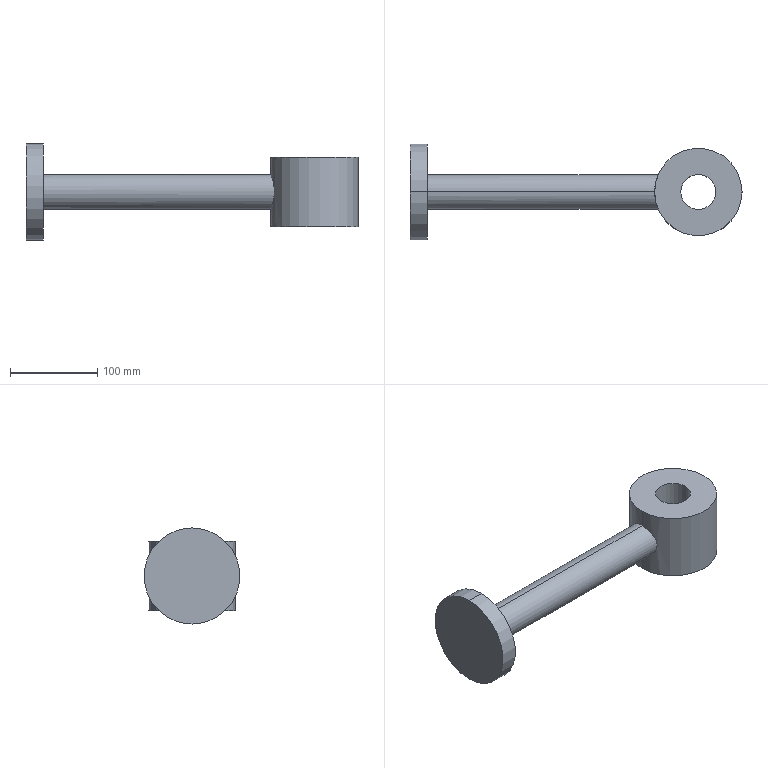Part | SolidWorks | 1 solid | 12 faces | box 380 x 110 x 110 mm | volume 1045872 mm3 | cylinder 8 | plane 4 | commonest cylinder face diameters 40 x4 100 x2 110 x2
STEP:
#1=CARTESIAN_POINT('',(310.,0.,40.));
#2=VERTEX_POINT('',#1);
#3=CARTESIAN_POINT('',(350.,0.,40.));
#4=VERTEX_POINT('',#3);
#5=CARTESIAN_POINT('',(330.,0.,40.));
#6=DIRECTION('',(0.,0.,1.));
#7=DIRECTION('',(1.,0.,0.));
#8=AXIS2_PLACEMENT_3D('',#5,#6,#7);
#9=CIRCLE('',#8,20.);
#10=EDGE_CURVE('',#2,#4,#9,.T.);
#11=ORIENTED_EDGE('',*,*,#10,.T.);
#12=CARTESIAN_POINT('',(350.,0.,-40.));
#13=VERTEX_POINT('',#12);
#14=CARTESIAN_POINT('',(350.,0.,40.));
#15=DIRECTION('',(0.,0.,-1.));
#16=VECTOR('',#15,1000.);
#17=LINE('',#14,#16);
#18=EDGE_CURVE('',#4,#13,#17,.T.);
#19=ORIENTED_EDGE('',*,*,#18,.T.);
#20=CARTESIAN_POINT('',(310.,0.,-40.));
#21=VERTEX_POINT('',#20);
#22=CARTESIAN_POINT('',(330.,0.,-40.));
#23=DIRECTION('',(0.,0.,1.));
#24=DIRECTION('',(1.,0.,0.));
#25=AXIS2_PLACEMENT_3D('',#22,#23,#24);
#26=CIRCLE('',#25,20.);
#27=EDGE_CURVE('',#21,#13,#26,.T.);
#28=ORIENTED_EDGE('',*,*,#27,.F.);
#29=CARTESIAN_POINT('',(310.,0.,40.));
#30=DIRECTION('',(0.,0.,-1.));
#31=VECTOR('',#30,1000.);
#32=LINE('',#29,#31);
#33=EDGE_CURVE('',#2,#21,#32,.T.);
#34=ORIENTED_EDGE('',*,*,#33,.F.);
#35=EDGE_LOOP('',(#11,#19,#28,#34));
#36=FACE_OUTER_BOUND('',#35,.T.);
#37=CARTESIAN_POINT('',(330.,0.,40.));
#38=DIRECTION('',(0.,0.,-1.));
#39=DIRECTION('',(-1.,0.,0.));
#40=AXIS2_PLACEMENT_3D('',#37,#38,#39);
#41=CYLINDRICAL_SURFACE('',#40,20.);
#42=ADVANCED_FACE('',(#36),#41,.F.);
#43=CARTESIAN_POINT('',(380.,0.,40.));
#44=VERTEX_POINT('',#43);
#45=CARTESIAN_POINT('',(280.,0.,40.));
#46=VERTEX_POINT('',#45);
#47=CARTESIAN_POINT('',(330.,0.,40.));
#48=DIRECTION('',(0.,0.,1.));
#49=DIRECTION('',(1.,0.,0.));
#50=AXIS2_PLACEMENT_3D('',#47,#48,#49);
#51=CIRCLE('',#50,50.);
#52=EDGE_CURVE('',#44,#46,#51,.T.);
#53=ORIENTED_EDGE('',*,*,#52,.F.);
#54=CARTESIAN_POINT('',(380.,0.,-40.));
#55=VERTEX_POINT('',#54);
#56=CARTESIAN_POINT('',(380.,0.,40.));
#57=DIRECTION('',(0.,0.,-1.));
#58=VECTOR('',#57,1000.);
#59=LINE('',#56,#58);
#60=EDGE_CURVE('',#44,#55,#59,.T.);
#61=ORIENTED_EDGE('',*,*,#60,.T.);
#62=CARTESIAN_POINT('',(280.,0.,-40.));
#63=VERTEX_POINT('',#62);
#64=CARTESIAN_POINT('',(330.,0.,-40.));
#65=DIRECTION('',(0.,0.,1.));
#66=DIRECTION('',(1.,0.,0.));
#67=AXIS2_PLACEMENT_3D('',#64,#65,#66);
#68=CIRCLE('',#67,50.);
#69=EDGE_CURVE('',#55,#63,#68,.T.);
#70=ORIENTED_EDGE('',*,*,#69,.T.);
#71=CARTESIAN_POINT('',(280.,0.,-20.));
#72=VERTEX_POINT('',#71);
#73=CARTESIAN_POINT('',(280.,0.,40.));
#74=DIRECTION('',(0.,0.,-1.));
#75=VECTOR('',#74,1000.);
#76=LINE('',#73,#75);
#77=EDGE_CURVE('',#72,#63,#76,.T.);
#78=ORIENTED_EDGE('',*,*,#77,.F.);
#79=CARTESIAN_POINT('',(280.,0.,20.));
#80=VERTEX_POINT('',#79);
#81=CARTESIAN_POINT('',(280.,0.,-20.));
#82=CARTESIAN_POINT('',(280.,0.6578,-20.));
#83=CARTESIAN_POINT('',(280.013,1.316,-19.968));
#84=CARTESIAN_POINT('',(280.065,2.635,-19.837));
#85=CARTESIAN_POINT('',(280.105,3.297,-19.737));
#86=CARTESIAN_POINT('',(280.258,5.241,-19.346));
#87=CARTESIAN_POINT('',(280.408,6.493,-18.962));
#88=CARTESIAN_POINT('',(280.691,8.307,-18.205));
#89=CARTESIAN_POINT('',(280.796,8.904,-17.92));
#90=CARTESIAN_POINT('',(281.018,10.058,-17.3));
#91=CARTESIAN_POINT('',(281.136,10.614,-16.963));
#92=CARTESIAN_POINT('',(281.383,11.69,-16.241));
#93=CARTESIAN_POINT('',(281.511,12.209,-15.855));
#94=CARTESIAN_POINT('',(281.774,13.209,-15.032));
#95=CARTESIAN_POINT('',(281.909,13.692,-14.593));
#96=CARTESIAN_POINT('',(282.317,15.074,-13.209));
#97=CARTESIAN_POINT('',(282.587,15.893,-12.211));
#98=CARTESIAN_POINT('',(282.967,16.972,-10.6));
#99=CARTESIAN_POINT('',(283.09,17.307,-10.044));
#100=CARTESIAN_POINT('',(283.323,17.926,-8.893));
#101=CARTESIAN_POINT('',(283.433,18.21,-8.296));
#102=CARTESIAN_POINT('',(283.733,18.964,-6.485));
#103=CARTESIAN_POINT('',(283.894,19.346,-5.239));
#104=CARTESIAN_POINT('',(284.06,19.736,-3.306));
#105=CARTESIAN_POINT('',(284.103,19.835,-2.649));
#106=CARTESIAN_POINT('',(284.16,19.967,-1.323));
#107=CARTESIAN_POINT('',(284.174,20.,-0.6615));
#108=CARTESIAN_POINT('',(284.174,20.,1.316));
#109=CARTESIAN_POINT('',(284.117,19.871,2.626));
#110=CARTESIAN_POINT('',(283.978,19.545,4.253));
#111=CARTESIAN_POINT('',(283.947,19.472,4.578));
#112=CARTESIAN_POINT('',(283.879,19.31,5.219));
#113=CARTESIAN_POINT('',(283.842,19.221,5.536));
#114=CARTESIAN_POINT('',(283.723,18.933,6.478));
#115=CARTESIAN_POINT('',(283.632,18.712,7.093));
#116=CARTESIAN_POINT('',(283.433,18.21,8.297));
#117=CARTESIAN_POINT('',(283.324,17.93,8.886));
#118=CARTESIAN_POINT('',(283.091,17.31,10.04));
#119=CARTESIAN_POINT('',(282.967,16.971,10.603));
#120=CARTESIAN_POINT('',(282.584,15.885,12.221));
#121=CARTESIAN_POINT('',(282.314,15.066,13.218));
#122=CARTESIAN_POINT('',(281.908,13.69,14.595));
#123=CARTESIAN_POINT('',(281.772,13.204,15.036));
#124=CARTESIAN_POINT('',(281.508,12.2,15.862));
#125=CARTESIAN_POINT('',(281.38,11.68,16.248));
#126=CARTESIAN_POINT('',(281.012,10.069,17.329));
#127=CARTESIAN_POINT('',(280.788,8.926,17.946));
#128=CARTESIAN_POINT('',(280.503,7.099,18.709));
#129=CARTESIAN_POINT('',(280.417,6.478,18.933));
#130=CARTESIAN_POINT('',(280.27,5.224,19.317));
#131=CARTESIAN_POINT('',(280.207,4.589,19.477));
#132=CARTESIAN_POINT('',(280.105,3.304,19.736));
#133=CARTESIAN_POINT('',(280.066,2.654,19.834));
#134=CARTESIAN_POINT('',(280.014,1.337,19.966));
#135=CARTESIAN_POINT('',(280.,0.6678,20.));
#136=CARTESIAN_POINT('',(280.,0.,20.));
#137=B_SPLINE_CURVE_WITH_KNOTS('',3,(#81,#82,#83,#84,#85,#86,#87,#88,#89,#90,#91,#92,#93,#94,#95,#96,#97,#98,#99,#100,#101,#102,#103,#104,#105,#106,#107,#108,#109,#110,#111,#112,#113,#114,#115,#116,#117,#118,#119,#120,#121,#122,#123,#124,#125,#126,#127,#128,#129,#130,#131,#132,#133,#134,#135,#136),.UNSPECIFIED.,.F.,.F.,(4,2,2,2,2,2,2,2,2,2,2,2,2,2,2,2,2,2,2,2,2,2,2,2,2,2,2,4),(0.0632,0.06517,0.06715,0.07109,0.07307,0.07504,0.07701,0.07899,0.08293,0.08491,0.08688,0.09083,0.0928,0.09478,0.09872,0.09971,0.1007,0.1027,0.1046,0.1066,0.1106,0.1125,0.1145,0.1185,0.1204,0.1224,0.1244,0.1264),.UNSPECIFIED.);
#138=EDGE_CURVE('',#72,#80,#137,.T.);
#139=ORIENTED_EDGE('',*,*,#138,.T.);
#140=CARTESIAN_POINT('',(280.,0.,40.));
#141=DIRECTION('',(0.,0.,-1.));
#142=VECTOR('',#141,1000.);
#143=LINE('',#140,#142);
#144=EDGE_CURVE('',#46,#80,#143,.T.);
#145=ORIENTED_EDGE('',*,*,#144,.F.);
#146=EDGE_LOOP('',(#53,#61,#70,#78,#139,#145));
#147=FACE_OUTER_BOUND('',#146,.T.);
#148=CARTESIAN_POINT('',(330.,0.,40.));
#149=DIRECTION('',(0.,0.,-1.));
#150=DIRECTION('',(-1.,0.,0.));
#151=AXIS2_PLACEMENT_3D('',#148,#149,#150);
#152=CYLINDRICAL_SURFACE('',#151,50.);
#153=ADVANCED_FACE('',(#147),#152,.T.);
#154=CARTESIAN_POINT('',(20.,0.,55.));
#155=VERTEX_POINT('',#154);
#156=CARTESIAN_POINT('',(20.,0.,-55.));
#157=VERTEX_POINT('',#156);
#158=CARTESIAN_POINT('',(20.,0.,0.));
#159=DIRECTION('',(-1.,0.,0.));
#160=DIRECTION('',(0.,0.,1.));
#161=AXIS2_PLACEMENT_3D('',#158,#159,#160);
#162=CIRCLE('',#161,55.);
#163=EDGE_CURVE('',#155,#157,#162,.T.);
#164=ORIENTED_EDGE('',*,*,#163,.T.);
#165=CARTESIAN_POINT('',(0.,0.,-55.));
#166=VERTEX_POINT('',#165);
#167=CARTESIAN_POINT('',(0.,0.,-55.));
#168=DIRECTION('',(-1.,0.,0.));
#169=VECTOR('',#168,1000.);
#170=LINE('',#167,#169);
#171=EDGE_CURVE('',#157,#166,#170,.T.);
#172=ORIENTED_EDGE('',*,*,#171,.T.);
#173=CARTESIAN_POINT('',(0.,0.,55.));
#174=VERTEX_POINT('',#173);
#175=CARTESIAN_POINT('',(0.,0.,0.));
#176=DIRECTION('',(-1.,0.,0.));
#177=DIRECTION('',(0.,0.,1.));
#178=AXIS2_PLACEMENT_3D('',#175,#176,#177);
#179=CIRCLE('',#178,55.);
#180=EDGE_CURVE('',#174,#166,#179,.T.);
#181=ORIENTED_EDGE('',*,*,#180,.F.);
#182=CARTESIAN_POINT('',(0.,0.,55.));
#183=DIRECTION('',(-1.,0.,0.));
#184=VECTOR('',#183,1000.);
#185=LINE('',#182,#184);
#186=EDGE_CURVE('',#155,#174,#185,.T.);
#187=ORIENTED_EDGE('',*,*,#186,.F.);
#188=EDGE_LOOP('',(#164,#172,#181,#187));
#189=FACE_OUTER_BOUND('',#188,.T.);
#190=CARTESIAN_POINT('',(0.,0.,0.));
#191=DIRECTION('',(-1.,0.,0.));
#192=DIRECTION('',(0.,0.,1.));
#193=AXIS2_PLACEMENT_3D('',#190,#191,#192);
#194=CYLINDRICAL_SURFACE('',#193,55.);
#195=ADVANCED_FACE('',(#189),#194,.T.);
#196=ORIENTED_EDGE('',*,*,#138,.F.);
#197=CARTESIAN_POINT('',(20.,0.,-20.));
#198=VERTEX_POINT('',#197);
#199=CARTESIAN_POINT('',(0.,0.,-20.));
#200=DIRECTION('',(-1.,0.,0.));
#201=VECTOR('',#200,1000.);
#202=LINE('',#199,#201);
#203=EDGE_CURVE('',#72,#198,#202,.T.);
#204=ORIENTED_EDGE('',*,*,#203,.T.);
#205=CARTESIAN_POINT('',(20.,0.,20.));
#206=VERTEX_POINT('',#205);
#207=CARTESIAN_POINT('',(20.,0.,0.));
#208=DIRECTION('',(-1.,0.,0.));
#209=DIRECTION('',(0.,0.,1.));
#210=AXIS2_PLACEMENT_3D('',#207,#208,#209);
#211=CIRCLE('',#210,20.);
#212=EDGE_CURVE('',#206,#198,#211,.T.);
#213=ORIENTED_EDGE('',*,*,#212,.F.);
#214=CARTESIAN_POINT('',(0.,0.,20.));
#215=DIRECTION('',(-1.,0.,0.));
#216=VECTOR('',#215,1000.);
#217=LINE('',#214,#216);
#218=EDGE_CURVE('',#80,#206,#217,.T.);
#219=ORIENTED_EDGE('',*,*,#218,.F.);
#220=EDGE_LOOP('',(#196,#204,#213,#219));
#221=FACE_OUTER_BOUND('',#220,.T.);
#222=CARTESIAN_POINT('',(0.,0.,0.));
#223=DIRECTION('',(-1.,0.,0.));
#224=DIRECTION('',(0.,0.,1.));
#225=AXIS2_PLACEMENT_3D('',#222,#223,#224);
#226=CYLINDRICAL_SURFACE('',#225,20.);
#227=ADVANCED_FACE('',(#221),#226,.T.);
#228=ORIENTED_EDGE('',*,*,#203,.F.);
#229=CARTESIAN_POINT('',(280.,0.,20.));
#230=CARTESIAN_POINT('',(280.,-1.337,20.));
#231=CARTESIAN_POINT('',(280.053,-2.648,19.867));
#232=CARTESIAN_POINT('',(280.206,-4.58,19.48));
#233=CARTESIAN_POINT('',(280.269,-5.218,19.319));
#234=CARTESIAN_POINT('',(280.381,-6.166,19.029));
#235=CARTESIAN_POINT('',(280.421,-6.482,18.923));
#236=CARTESIAN_POINT('',(280.506,-7.102,18.699));
#237=CARTESIAN_POINT('',(280.551,-7.409,18.58));
#238=CARTESIAN_POINT('',(280.787,-8.919,17.949));
#239=CARTESIAN_POINT('',(281.011,-10.063,17.333));
#240=CARTESIAN_POINT('',(281.382,-11.686,16.244));
#241=CARTESIAN_POINT('',(281.512,-12.213,15.851));
#242=CARTESIAN_POINT('',(281.776,-13.217,15.025));
#243=CARTESIAN_POINT('',(281.91,-13.695,14.59));
#244=CARTESIAN_POINT('',(282.179,-14.607,13.677));
#245=CARTESIAN_POINT('',(282.314,-15.04,13.199));
#246=CARTESIAN_POINT('',(282.581,-15.862,12.199));
#247=CARTESIAN_POINT('',(282.713,-16.252,11.675));
#248=CARTESIAN_POINT('',(283.098,-17.344,10.045));
#249=CARTESIAN_POINT('',(283.333,-17.957,8.902));
#250=CARTESIAN_POINT('',(283.631,-18.708,7.102));
#251=CARTESIAN_POINT('',(283.722,-18.93,6.488));
#252=CARTESIAN_POINT('',(283.881,-19.316,5.228));
#253=CARTESIAN_POINT('',(283.95,-19.479,4.581));
#254=CARTESIAN_POINT('',(284.116,-19.869,2.64));
#255=CARTESIAN_POINT('',(284.174,-19.999,1.333));
#256=CARTESIAN_POINT('',(284.174,-20.,-0.3179));
#257=CARTESIAN_POINT('',(284.171,-19.992,-0.6489));
#258=CARTESIAN_POINT('',(284.157,-19.96,-1.313));
#259=CARTESIAN_POINT('',(284.146,-19.935,-1.646));
#260=CARTESIAN_POINT('',(284.103,-19.836,-2.64));
#261=CARTESIAN_POINT('',(284.061,-19.738,-3.293));
#262=CARTESIAN_POINT('',(283.895,-19.35,-5.227));
#263=CARTESIAN_POINT('',(283.734,-18.966,-6.483));
#264=CARTESIAN_POINT('',(283.33,-17.95,-8.919));
#265=CARTESIAN_POINT('',(283.094,-17.332,-10.063));
#266=CARTESIAN_POINT('',(282.713,-16.25,-11.678));
#267=CARTESIAN_POINT('',(282.581,-15.862,-12.199));
#268=CARTESIAN_POINT('',(282.312,-15.034,-13.207));
#269=CARTESIAN_POINT('',(282.175,-14.595,-13.69));
#270=CARTESIAN_POINT('',(281.77,-13.221,-15.062));
#271=CARTESIAN_POINT('',(281.505,-12.225,-15.882));
#272=CARTESIAN_POINT('',(281.134,-10.604,-16.97));
#273=CARTESIAN_POINT('',(281.015,-10.039,-17.31));
#274=CARTESIAN_POINT('',(280.792,-8.886,-17.93));
#275=CARTESIAN_POINT('',(280.689,-8.297,-18.209));
#276=CARTESIAN_POINT('',(280.409,-6.494,-18.961));
#277=CARTESIAN_POINT('',(280.258,-5.243,-19.346));
#278=CARTESIAN_POINT('',(280.13,-3.614,-19.674));
#279=CARTESIAN_POINT('',(280.107,-3.285,-19.731));
#280=CARTESIAN_POINT('',(280.068,-2.629,-19.829));
#281=CARTESIAN_POINT('',(280.052,-2.301,-19.87));
#282=CARTESIAN_POINT('',(280.013,-1.316,-19.968));
#283=CARTESIAN_POINT('',(280.,-0.6582,-20.));
#284=CARTESIAN_POINT('',(280.,0.,-20.));
#285=B_SPLINE_CURVE_WITH_KNOTS('',3,(#229,#230,#231,#232,#233,#234,#235,#236,#237,#238,#239,#240,#241,#242,#243,#244,#245,#246,#247,#248,#249,#250,#251,#252,#253,#254,#255,#256,#257,#258,#259,#260,#261,#262,#263,#264,#265,#266,#267,#268,#269,#270,#271,#272,#273,#274,#275,#276,#277,#278,#279,#280,#281,#282,#283,#284),.UNSPECIFIED.,.F.,.F.,(4,2,2,2,2,2,2,2,2,2,2,2,2,2,2,2,2,2,2,2,2,2,2,2,2,2,2,4),(0.,0.00395,0.005925,0.006912,0.0079,0.01185,0.01382,0.0158,0.01777,0.01975,0.0237,0.02567,0.02765,0.0316,0.03259,0.03357,0.03555,0.0395,0.04345,0.04542,0.0474,0.05135,0.05332,0.0553,0.05925,0.06024,0.06122,0.0632),.UNSPECIFIED.);
#286=EDGE_CURVE('',#80,#72,#285,.T.);
#287=ORIENTED_EDGE('',*,*,#286,.F.);
#288=ORIENTED_EDGE('',*,*,#218,.T.);
#289=CARTESIAN_POINT('',(20.,0.,0.));
#290=DIRECTION('',(-1.,0.,0.));
#291=DIRECTION('',(0.,0.,1.));
#292=AXIS2_PLACEMENT_3D('',#289,#290,#291);
#293=CIRCLE('',#292,20.);
#294=EDGE_CURVE('',#198,#206,#293,.T.);
#295=ORIENTED_EDGE('',*,*,#294,.F.);
#296=EDGE_LOOP('',(#228,#287,#288,#295));
#297=FACE_OUTER_BOUND('',#296,.T.);
#298=CARTESIAN_POINT('',(0.,0.,0.));
#299=DIRECTION('',(-1.,0.,0.));
#300=DIRECTION('',(0.,0.,1.));
#301=AXIS2_PLACEMENT_3D('',#298,#299,#300);
#302=CYLINDRICAL_SURFACE('',#301,20.);
#303=ADVANCED_FACE('',(#297),#302,.T.);
#304=ORIENTED_EDGE('',*,*,#163,.F.);
#305=CARTESIAN_POINT('',(20.,0.,0.));
#306=DIRECTION('',(-1.,0.,0.));
#307=DIRECTION('',(0.,0.,1.));
#308=AXIS2_PLACEMENT_3D('',#305,#306,#307);
#309=CIRCLE('',#308,55.);
#310=EDGE_CURVE('',#157,#155,#309,.T.);
#311=ORIENTED_EDGE('',*,*,#310,.F.);
#312=EDGE_LOOP('',(#304,#311));
#313=FACE_OUTER_BOUND('',#312,.T.);
#314=ORIENTED_EDGE('',*,*,#212,.T.);
#315=ORIENTED_EDGE('',*,*,#294,.T.);
#316=EDGE_LOOP('',(#314,#315));
#317=FACE_BOUND('',#316,.T.);
#318=CARTESIAN_POINT('',(20.,20.,0.));
#319=DIRECTION('',(-1.,0.,0.));
#320=DIRECTION('',(0.,0.,1.));
#321=AXIS2_PLACEMENT_3D('',#318,#319,#320);
#322=PLANE('',#321);
#323=ADVANCED_FACE('',(#313,#317),#322,.F.);
#324=ORIENTED_EDGE('',*,*,#171,.F.);
#325=ORIENTED_EDGE('',*,*,#310,.T.);
#326=ORIENTED_EDGE('',*,*,#186,.T.);
#327=CARTESIAN_POINT('',(0.,0.,0.));
#328=DIRECTION('',(-1.,0.,0.));
#329=DIRECTION('',(0.,0.,1.));
#330=AXIS2_PLACEMENT_3D('',#327,#328,#329);
#331=CIRCLE('',#330,55.);
#332=EDGE_CURVE('',#166,#174,#331,.T.);
#333=ORIENTED_EDGE('',*,*,#332,.F.);
#334=EDGE_LOOP('',(#324,#325,#326,#333));
#335=FACE_OUTER_BOUND('',#334,.T.);
#336=CARTESIAN_POINT('',(0.,0.,0.));
#337=DIRECTION('',(-1.,0.,0.));
#338=DIRECTION('',(0.,0.,1.));
#339=AXIS2_PLACEMENT_3D('',#336,#337,#338);
#340=CYLINDRICAL_SURFACE('',#339,55.);
#341=ADVANCED_FACE('',(#335),#340,.T.);
#342=ORIENTED_EDGE('',*,*,#180,.T.);
#343=ORIENTED_EDGE('',*,*,#332,.T.);
#344=EDGE_LOOP('',(#342,#343));
#345=FACE_OUTER_BOUND('',#344,.T.);
#346=CARTESIAN_POINT('',(0.,55.,0.));
#347=DIRECTION('',(1.,0.,0.));
#348=DIRECTION('',(0.,0.,-1.));
#349=AXIS2_PLACEMENT_3D('',#346,#347,#348);
#350=PLANE('',#349);
#351=ADVANCED_FACE('',(#345),#350,.F.);
#352=ORIENTED_EDGE('',*,*,#60,.F.);
#353=CARTESIAN_POINT('',(330.,0.,40.));
#354=DIRECTION('',(0.,0.,1.));
#355=DIRECTION('',(1.,0.,0.));
#356=AXIS2_PLACEMENT_3D('',#353,#354,#355);
#357=CIRCLE('',#356,50.);
#358=EDGE_CURVE('',#46,#44,#357,.T.);
#359=ORIENTED_EDGE('',*,*,#358,.F.);
#360=ORIENTED_EDGE('',*,*,#144,.T.);
#361=ORIENTED_EDGE('',*,*,#286,.T.);
#362=ORIENTED_EDGE('',*,*,#77,.T.);
#363=CARTESIAN_POINT('',(330.,0.,-40.));
#364=DIRECTION('',(0.,0.,1.));
#365=DIRECTION('',(1.,0.,0.));
#366=AXIS2_PLACEMENT_3D('',#363,#364,#365);
#367=CIRCLE('',#366,50.);
#368=EDGE_CURVE('',#63,#55,#367,.T.);
#369=ORIENTED_EDGE('',*,*,#368,.T.);
#370=EDGE_LOOP('',(#352,#359,#360,#361,#362,#369));
#371=FACE_OUTER_BOUND('',#370,.T.);
#372=CARTESIAN_POINT('',(330.,0.,40.));
#373=DIRECTION('',(0.,0.,-1.));
#374=DIRECTION('',(-1.,0.,0.));
#375=AXIS2_PLACEMENT_3D('',#372,#373,#374);
#376=CYLINDRICAL_SURFACE('',#375,50.);
#377=ADVANCED_FACE('',(#371),#376,.T.);
#378=ORIENTED_EDGE('',*,*,#358,.T.);
#379=ORIENTED_EDGE('',*,*,#52,.T.);
#380=EDGE_LOOP('',(#378,#379));
#381=FACE_OUTER_BOUND('',#380,.T.);
#382=ORIENTED_EDGE('',*,*,#10,.F.);
#383=CARTESIAN_POINT('',(330.,0.,40.));
#384=DIRECTION('',(0.,0.,1.));
#385=DIRECTION('',(1.,0.,0.));
#386=AXIS2_PLACEMENT_3D('',#383,#384,#385);
#387=CIRCLE('',#386,20.);
#388=EDGE_CURVE('',#4,#2,#387,.T.);
#389=ORIENTED_EDGE('',*,*,#388,.F.);
#390=EDGE_LOOP('',(#382,#389));
#391=FACE_BOUND('',#390,.T.);
#392=CARTESIAN_POINT('',(330.,0.,40.));
#393=DIRECTION('',(0.,0.,1.));
#394=DIRECTION('',(1.,0.,0.));
#395=AXIS2_PLACEMENT_3D('',#392,#393,#394);
#396=PLANE('',#395);
#397=ADVANCED_FACE('',(#381,#391),#396,.T.);
#398=ORIENTED_EDGE('',*,*,#368,.F.);
#399=ORIENTED_EDGE('',*,*,#69,.F.);
#400=EDGE_LOOP('',(#398,#399));
#401=FACE_OUTER_BOUND('',#400,.T.);
#402=ORIENTED_EDGE('',*,*,#27,.T.);
#403=CARTESIAN_POINT('',(330.,0.,-40.));
#404=DIRECTION('',(0.,0.,1.));
#405=DIRECTION('',(1.,0.,0.));
#406=AXIS2_PLACEMENT_3D('',#403,#404,#405);
#407=CIRCLE('',#406,20.);
#408=EDGE_CURVE('',#13,#21,#407,.T.);
#409=ORIENTED_EDGE('',*,*,#408,.T.);
#410=EDGE_LOOP('',(#402,#409));
#411=FACE_BOUND('',#410,.T.);
#412=CARTESIAN_POINT('',(330.,0.,-40.));
#413=DIRECTION('',(0.,0.,1.));
#414=DIRECTION('',(1.,0.,0.));
#415=AXIS2_PLACEMENT_3D('',#412,#413,#414);
#416=PLANE('',#415);
#417=ADVANCED_FACE('',(#401,#411),#416,.F.);
#418=ORIENTED_EDGE('',*,*,#18,.F.);
#419=ORIENTED_EDGE('',*,*,#388,.T.);
#420=ORIENTED_EDGE('',*,*,#33,.T.);
#421=ORIENTED_EDGE('',*,*,#408,.F.);
#422=EDGE_LOOP('',(#418,#419,#420,#421));
#423=FACE_OUTER_BOUND('',#422,.T.);
#424=CARTESIAN_POINT('',(330.,0.,40.));
#425=DIRECTION('',(0.,0.,-1.));
#426=DIRECTION('',(-1.,0.,0.));
#427=AXIS2_PLACEMENT_3D('',#424,#425,#426);
#428=CYLINDRICAL_SURFACE('',#427,20.);
#429=ADVANCED_FACE('',(#423),#428,.F.);
#430=CLOSED_SHELL('',(#42,#153,#195,#227,#303,#323,#341,#351,#377,#397,#417,#429));
#431=MANIFOLD_SOLID_BREP('',#430);
#432=CARTESIAN_POINT('',(0.,0.,0.));
#433=DIRECTION('',(0.,0.,1.));
#434=DIRECTION('',(1.,0.,0.));
#435=AXIS2_PLACEMENT_3D('',#432,#433,#434);
#436=(LENGTH_UNIT()NAMED_UNIT(*)SI_UNIT(.MILLI.,.METRE.));
#437=UNCERTAINTY_MEASURE_WITH_UNIT(LENGTH_MEASURE(0.00001),#436,'','');
#438=(NAMED_UNIT(*)PLANE_ANGLE_UNIT()SI_UNIT($,.RADIAN.));
#439=(NAMED_UNIT(*)SI_UNIT($,.STERADIAN.)SOLID_ANGLE_UNIT());
#440=(GEOMETRIC_REPRESENTATION_CONTEXT(3)GLOBAL_UNCERTAINTY_ASSIGNED_CONTEXT((#437))GLOBAL_UNIT_ASSIGNED_CONTEXT((#436,#438,#439))REPRESENTATION_CONTEXT('',''));
#441=ADVANCED_BREP_SHAPE_REPRESENTATION('',(#431,#435),#440);